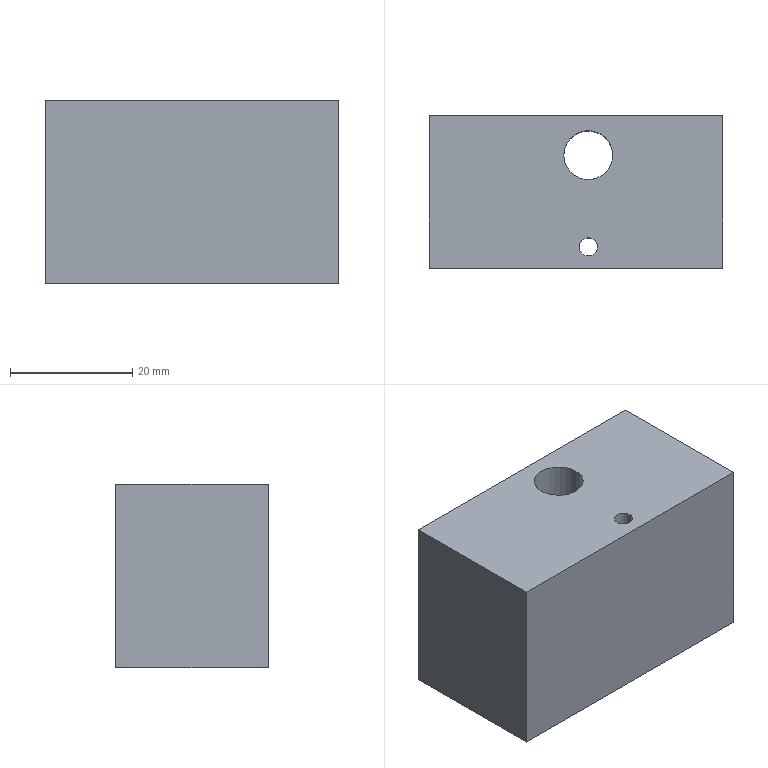Part | SolidWorks | features Cut 2, Extrusion 1, HoleWzd 1 | 1 solid | 22 faces | box 48 x 25 x 30 mm | volume 34166 mm3 | cylinder 10 | cone 6 | plane 6 | commonest cylinder face diameters 2.5 x6 3 x2 8 x2
STEP:
#1=CARTESIAN_POINT('',(12.5,17.5,-12.75));
#2=VERTEX_POINT('',#1);
#3=CARTESIAN_POINT('',(12.5,17.5,-10.25));
#4=VERTEX_POINT('',#3);
#5=CARTESIAN_POINT('',(12.5,17.5,-11.5));
#6=DIRECTION('',(0.,1.,0.));
#7=DIRECTION('',(0.,0.,1.));
#8=AXIS2_PLACEMENT_3D('',#5,#6,#7);
#9=CIRCLE('',#8,1.25);
#10=EDGE_CURVE('',#2,#4,#9,.T.);
#11=ORIENTED_EDGE('',*,*,#10,.F.);
#12=CARTESIAN_POINT('',(12.5,25.,-12.75));
#13=VERTEX_POINT('',#12);
#14=CARTESIAN_POINT('',(12.5,25.,-12.75));
#15=DIRECTION('',(0.,1.,0.));
#16=VECTOR('',#15,1000.);
#17=LINE('',#14,#16);
#18=EDGE_CURVE('',#2,#13,#17,.T.);
#19=ORIENTED_EDGE('',*,*,#18,.T.);
#20=CARTESIAN_POINT('',(12.5,25.,-10.25));
#21=VERTEX_POINT('',#20);
#22=CARTESIAN_POINT('',(12.5,25.,-11.5));
#23=DIRECTION('',(0.,1.,0.));
#24=DIRECTION('',(0.,0.,1.));
#25=AXIS2_PLACEMENT_3D('',#22,#23,#24);
#26=CIRCLE('',#25,1.25);
#27=EDGE_CURVE('',#13,#21,#26,.T.);
#28=ORIENTED_EDGE('',*,*,#27,.T.);
#29=CARTESIAN_POINT('',(12.5,25.,-10.25));
#30=DIRECTION('',(0.,1.,0.));
#31=VECTOR('',#30,1000.);
#32=LINE('',#29,#31);
#33=EDGE_CURVE('',#4,#21,#32,.T.);
#34=ORIENTED_EDGE('',*,*,#33,.F.);
#35=EDGE_LOOP('',(#11,#19,#28,#34));
#36=FACE_OUTER_BOUND('',#35,.T.);
#37=CARTESIAN_POINT('',(12.5,25.,-11.5));
#38=DIRECTION('',(0.,1.,0.));
#39=DIRECTION('',(0.,0.,1.));
#40=AXIS2_PLACEMENT_3D('',#37,#38,#39);
#41=CYLINDRICAL_SURFACE('',#40,1.25);
#42=ADVANCED_FACE('',(#36),#41,.F.);
#43=CARTESIAN_POINT('',(12.5,16.749,-11.5));
#44=VERTEX_POINT('',#43);
#45=CARTESIAN_POINT('',(12.5,17.5,-10.25));
#46=DIRECTION('',(0.,0.515,0.8572));
#47=VECTOR('',#46,1000.);
#48=LINE('',#45,#47);
#49=EDGE_CURVE('',#44,#4,#48,.T.);
#50=ORIENTED_EDGE('',*,*,#49,.F.);
#51=CARTESIAN_POINT('',(12.5,17.5,-12.75));
#52=DIRECTION('',(0.,0.515,-0.8572));
#53=VECTOR('',#52,1000.);
#54=LINE('',#51,#53);
#55=EDGE_CURVE('',#44,#2,#54,.T.);
#56=ORIENTED_EDGE('',*,*,#55,.T.);
#57=ORIENTED_EDGE('',*,*,#10,.T.);
#58=EDGE_LOOP('',(#50,#56,#57));
#59=FACE_OUTER_BOUND('',#58,.T.);
#60=CARTESIAN_POINT('',(12.5,17.5,-11.5));
#61=DIRECTION('',(0.,1.,0.));
#62=DIRECTION('',(0.,0.,1.));
#63=AXIS2_PLACEMENT_3D('',#60,#61,#62);
#64=CONICAL_SURFACE('',#63,1.25,1.03);
#65=ADVANCED_FACE('',(#59),#64,.F.);
#66=CARTESIAN_POINT('',(12.5,17.5,-1.25));
#67=VERTEX_POINT('',#66);
#68=CARTESIAN_POINT('',(12.5,17.5,1.25));
#69=VERTEX_POINT('',#68);
#70=CARTESIAN_POINT('',(12.5,17.5,0.));
#71=DIRECTION('',(0.,1.,0.));
#72=DIRECTION('',(0.,0.,1.));
#73=AXIS2_PLACEMENT_3D('',#70,#71,#72);
#74=CIRCLE('',#73,1.25);
#75=EDGE_CURVE('',#67,#69,#74,.T.);
#76=ORIENTED_EDGE('',*,*,#75,.F.);
#77=CARTESIAN_POINT('',(12.5,25.,-1.25));
#78=VERTEX_POINT('',#77);
#79=CARTESIAN_POINT('',(12.5,25.,-1.25));
#80=DIRECTION('',(0.,1.,0.));
#81=VECTOR('',#80,1000.);
#82=LINE('',#79,#81);
#83=EDGE_CURVE('',#67,#78,#82,.T.);
#84=ORIENTED_EDGE('',*,*,#83,.T.);
#85=CARTESIAN_POINT('',(12.5,25.,1.25));
#86=VERTEX_POINT('',#85);
#87=CARTESIAN_POINT('',(12.5,25.,0.));
#88=DIRECTION('',(0.,1.,0.));
#89=DIRECTION('',(0.,0.,1.));
#90=AXIS2_PLACEMENT_3D('',#87,#88,#89);
#91=CIRCLE('',#90,1.25);
#92=EDGE_CURVE('',#78,#86,#91,.T.);
#93=ORIENTED_EDGE('',*,*,#92,.T.);
#94=CARTESIAN_POINT('',(12.5,25.,1.25));
#95=DIRECTION('',(0.,1.,0.));
#96=VECTOR('',#95,1000.);
#97=LINE('',#94,#96);
#98=EDGE_CURVE('',#69,#86,#97,.T.);
#99=ORIENTED_EDGE('',*,*,#98,.F.);
#100=EDGE_LOOP('',(#76,#84,#93,#99));
#101=FACE_OUTER_BOUND('',#100,.T.);
#102=CARTESIAN_POINT('',(12.5,25.,0.));
#103=DIRECTION('',(0.,1.,0.));
#104=DIRECTION('',(0.,0.,1.));
#105=AXIS2_PLACEMENT_3D('',#102,#103,#104);
#106=CYLINDRICAL_SURFACE('',#105,1.25);
#107=ADVANCED_FACE('',(#101),#106,.F.);
#108=CARTESIAN_POINT('',(12.5,16.749,0.));
#109=VERTEX_POINT('',#108);
#110=CARTESIAN_POINT('',(12.5,17.5,1.25));
#111=DIRECTION('',(0.,0.515,0.8572));
#112=VECTOR('',#111,1000.);
#113=LINE('',#110,#112);
#114=EDGE_CURVE('',#109,#69,#113,.T.);
#115=ORIENTED_EDGE('',*,*,#114,.F.);
#116=CARTESIAN_POINT('',(12.5,17.5,-1.25));
#117=DIRECTION('',(0.,0.515,-0.8572));
#118=VECTOR('',#117,1000.);
#119=LINE('',#116,#118);
#120=EDGE_CURVE('',#109,#67,#119,.T.);
#121=ORIENTED_EDGE('',*,*,#120,.T.);
#122=ORIENTED_EDGE('',*,*,#75,.T.);
#123=EDGE_LOOP('',(#115,#121,#122));
#124=FACE_OUTER_BOUND('',#123,.T.);
#125=CARTESIAN_POINT('',(12.5,17.5,0.));
#126=DIRECTION('',(0.,1.,0.));
#127=DIRECTION('',(0.,0.,1.));
#128=AXIS2_PLACEMENT_3D('',#125,#126,#127);
#129=CONICAL_SURFACE('',#128,1.25,1.03);
#130=ADVANCED_FACE('',(#124),#129,.F.);
#131=CARTESIAN_POINT('',(12.5,17.5,10.25));
#132=VERTEX_POINT('',#131);
#133=CARTESIAN_POINT('',(12.5,17.5,12.75));
#134=VERTEX_POINT('',#133);
#135=CARTESIAN_POINT('',(12.5,17.5,11.5));
#136=DIRECTION('',(0.,1.,0.));
#137=DIRECTION('',(0.,0.,1.));
#138=AXIS2_PLACEMENT_3D('',#135,#136,#137);
#139=CIRCLE('',#138,1.25);
#140=EDGE_CURVE('',#132,#134,#139,.T.);
#141=ORIENTED_EDGE('',*,*,#140,.F.);
#142=CARTESIAN_POINT('',(12.5,25.,10.25));
#143=VERTEX_POINT('',#142);
#144=CARTESIAN_POINT('',(12.5,25.,10.25));
#145=DIRECTION('',(0.,1.,0.));
#146=VECTOR('',#145,1000.);
#147=LINE('',#144,#146);
#148=EDGE_CURVE('',#132,#143,#147,.T.);
#149=ORIENTED_EDGE('',*,*,#148,.T.);
#150=CARTESIAN_POINT('',(12.5,25.,12.75));
#151=VERTEX_POINT('',#150);
#152=CARTESIAN_POINT('',(12.5,25.,11.5));
#153=DIRECTION('',(0.,1.,0.));
#154=DIRECTION('',(0.,0.,1.));
#155=AXIS2_PLACEMENT_3D('',#152,#153,#154);
#156=CIRCLE('',#155,1.25);
#157=EDGE_CURVE('',#143,#151,#156,.T.);
#158=ORIENTED_EDGE('',*,*,#157,.T.);
#159=CARTESIAN_POINT('',(12.5,25.,12.75));
#160=DIRECTION('',(0.,1.,0.));
#161=VECTOR('',#160,1000.);
#162=LINE('',#159,#161);
#163=EDGE_CURVE('',#134,#151,#162,.T.);
#164=ORIENTED_EDGE('',*,*,#163,.F.);
#165=EDGE_LOOP('',(#141,#149,#158,#164));
#166=FACE_OUTER_BOUND('',#165,.T.);
#167=CARTESIAN_POINT('',(12.5,25.,11.5));
#168=DIRECTION('',(0.,1.,0.));
#169=DIRECTION('',(0.,0.,1.));
#170=AXIS2_PLACEMENT_3D('',#167,#168,#169);
#171=CYLINDRICAL_SURFACE('',#170,1.25);
#172=ADVANCED_FACE('',(#166),#171,.F.);
#173=CARTESIAN_POINT('',(12.5,16.749,11.5));
#174=VERTEX_POINT('',#173);
#175=CARTESIAN_POINT('',(12.5,17.5,12.75));
#176=DIRECTION('',(0.,0.515,0.8572));
#177=VECTOR('',#176,1000.);
#178=LINE('',#175,#177);
#179=EDGE_CURVE('',#174,#134,#178,.T.);
#180=ORIENTED_EDGE('',*,*,#179,.F.);
#181=CARTESIAN_POINT('',(12.5,17.5,10.25));
#182=DIRECTION('',(0.,0.515,-0.8572));
#183=VECTOR('',#182,1000.);
#184=LINE('',#181,#183);
#185=EDGE_CURVE('',#174,#132,#184,.T.);
#186=ORIENTED_EDGE('',*,*,#185,.T.);
#187=ORIENTED_EDGE('',*,*,#140,.T.);
#188=EDGE_LOOP('',(#180,#186,#187));
#189=FACE_OUTER_BOUND('',#188,.T.);
#190=CARTESIAN_POINT('',(12.5,17.5,11.5));
#191=DIRECTION('',(0.,1.,0.));
#192=DIRECTION('',(0.,0.,1.));
#193=AXIS2_PLACEMENT_3D('',#190,#191,#192);
#194=CONICAL_SURFACE('',#193,1.25,1.03);
#195=ADVANCED_FACE('',(#189),#194,.F.);
#196=CARTESIAN_POINT('',(6.,18.5,-15.));
#197=VERTEX_POINT('',#196);
#198=CARTESIAN_POINT('',(-2.,18.5,-15.));
#199=VERTEX_POINT('',#198);
#200=CARTESIAN_POINT('',(2.,18.5,-15.));
#201=DIRECTION('',(0.,0.,-1.));
#202=DIRECTION('',(1.,0.,0.));
#203=AXIS2_PLACEMENT_3D('',#200,#201,#202);
#204=CIRCLE('',#203,4.);
#205=EDGE_CURVE('',#197,#199,#204,.T.);
#206=ORIENTED_EDGE('',*,*,#205,.T.);
#207=CARTESIAN_POINT('',(-2.,18.5,15.));
#208=VERTEX_POINT('',#207);
#209=CARTESIAN_POINT('',(-2.,18.5,-15.001));
#210=DIRECTION('',(0.,0.,1.));
#211=VECTOR('',#210,1000.);
#212=LINE('',#209,#211);
#213=EDGE_CURVE('',#199,#208,#212,.T.);
#214=ORIENTED_EDGE('',*,*,#213,.T.);
#215=CARTESIAN_POINT('',(6.,18.5,15.));
#216=VERTEX_POINT('',#215);
#217=CARTESIAN_POINT('',(2.,18.5,15.));
#218=DIRECTION('',(0.,0.,1.));
#219=DIRECTION('',(1.,0.,0.));
#220=AXIS2_PLACEMENT_3D('',#217,#218,#219);
#221=CIRCLE('',#220,4.);
#222=EDGE_CURVE('',#208,#216,#221,.T.);
#223=ORIENTED_EDGE('',*,*,#222,.T.);
#224=CARTESIAN_POINT('',(6.,18.5,-15.001));
#225=DIRECTION('',(0.,0.,1.));
#226=VECTOR('',#225,1000.);
#227=LINE('',#224,#226);
#228=EDGE_CURVE('',#197,#216,#227,.T.);
#229=ORIENTED_EDGE('',*,*,#228,.F.);
#230=EDGE_LOOP('',(#206,#214,#223,#229));
#231=FACE_OUTER_BOUND('',#230,.T.);
#232=CARTESIAN_POINT('',(2.,18.5,-15.001));
#233=DIRECTION('',(0.,0.,1.));
#234=DIRECTION('',(1.,0.,0.));
#235=AXIS2_PLACEMENT_3D('',#232,#233,#234);
#236=CYLINDRICAL_SURFACE('',#235,4.);
#237=ADVANCED_FACE('',(#231),#236,.F.);
#238=CARTESIAN_POINT('',(3.5,3.5,-15.));
#239=VERTEX_POINT('',#238);
#240=CARTESIAN_POINT('',(0.5,3.5,-15.));
#241=VERTEX_POINT('',#240);
#242=CARTESIAN_POINT('',(2.,3.5,-15.));
#243=DIRECTION('',(0.,0.,-1.));
#244=DIRECTION('',(1.,0.,0.));
#245=AXIS2_PLACEMENT_3D('',#242,#243,#244);
#246=CIRCLE('',#245,1.5);
#247=EDGE_CURVE('',#239,#241,#246,.T.);
#248=ORIENTED_EDGE('',*,*,#247,.T.);
#249=CARTESIAN_POINT('',(0.5,3.5,15.));
#250=VERTEX_POINT('',#249);
#251=CARTESIAN_POINT('',(0.5,3.5,-15.001));
#252=DIRECTION('',(0.,0.,1.));
#253=VECTOR('',#252,1000.);
#254=LINE('',#251,#253);
#255=EDGE_CURVE('',#241,#250,#254,.T.);
#256=ORIENTED_EDGE('',*,*,#255,.T.);
#257=CARTESIAN_POINT('',(3.5,3.5,15.));
#258=VERTEX_POINT('',#257);
#259=CARTESIAN_POINT('',(2.,3.5,15.));
#260=DIRECTION('',(0.,0.,1.));
#261=DIRECTION('',(1.,0.,0.));
#262=AXIS2_PLACEMENT_3D('',#259,#260,#261);
#263=CIRCLE('',#262,1.5);
#264=EDGE_CURVE('',#250,#258,#263,.T.);
#265=ORIENTED_EDGE('',*,*,#264,.T.);
#266=CARTESIAN_POINT('',(3.5,3.5,-15.001));
#267=DIRECTION('',(0.,0.,1.));
#268=VECTOR('',#267,1000.);
#269=LINE('',#266,#268);
#270=EDGE_CURVE('',#239,#258,#269,.T.);
#271=ORIENTED_EDGE('',*,*,#270,.F.);
#272=EDGE_LOOP('',(#248,#256,#265,#271));
#273=FACE_OUTER_BOUND('',#272,.T.);
#274=CARTESIAN_POINT('',(2.,3.5,-15.001));
#275=DIRECTION('',(0.,0.,1.));
#276=DIRECTION('',(1.,0.,0.));
#277=AXIS2_PLACEMENT_3D('',#274,#275,#276);
#278=CYLINDRICAL_SURFACE('',#277,1.5);
#279=ADVANCED_FACE('',(#273),#278,.F.);
#280=CARTESIAN_POINT('',(24.,0.,15.));
#281=VERTEX_POINT('',#280);
#282=CARTESIAN_POINT('',(24.,0.,-15.));
#283=VERTEX_POINT('',#282);
#284=CARTESIAN_POINT('',(24.,0.,-15.));
#285=DIRECTION('',(0.,0.,-1.));
#286=VECTOR('',#285,1000.);
#287=LINE('',#284,#286);
#288=EDGE_CURVE('',#281,#283,#287,.T.);
#289=ORIENTED_EDGE('',*,*,#288,.T.);
#290=CARTESIAN_POINT('',(24.,25.,-15.));
#291=VERTEX_POINT('',#290);
#292=CARTESIAN_POINT('',(24.,25.,-15.));
#293=DIRECTION('',(0.,-1.,0.));
#294=VECTOR('',#293,1000.);
#295=LINE('',#292,#294);
#296=EDGE_CURVE('',#291,#283,#295,.T.);
#297=ORIENTED_EDGE('',*,*,#296,.F.);
#298=CARTESIAN_POINT('',(24.,25.,15.));
#299=VERTEX_POINT('',#298);
#300=CARTESIAN_POINT('',(24.,25.,-15.));
#301=DIRECTION('',(0.,0.,-1.));
#302=VECTOR('',#301,1000.);
#303=LINE('',#300,#302);
#304=EDGE_CURVE('',#299,#291,#303,.T.);
#305=ORIENTED_EDGE('',*,*,#304,.F.);
#306=CARTESIAN_POINT('',(24.,25.,15.));
#307=DIRECTION('',(0.,-1.,0.));
#308=VECTOR('',#307,1000.);
#309=LINE('',#306,#308);
#310=EDGE_CURVE('',#299,#281,#309,.T.);
#311=ORIENTED_EDGE('',*,*,#310,.T.);
#312=EDGE_LOOP('',(#289,#297,#305,#311));
#313=FACE_OUTER_BOUND('',#312,.T.);
#314=CARTESIAN_POINT('',(24.,25.,-15.));
#315=DIRECTION('',(-1.,0.,0.));
#316=DIRECTION('',(0.,0.,1.));
#317=AXIS2_PLACEMENT_3D('',#314,#315,#316);
#318=PLANE('',#317);
#319=ADVANCED_FACE('',(#313),#318,.F.);
#320=ORIENTED_EDGE('',*,*,#205,.F.);
#321=CARTESIAN_POINT('',(2.,18.5,-15.));
#322=DIRECTION('',(0.,0.,-1.));
#323=DIRECTION('',(1.,0.,0.));
#324=AXIS2_PLACEMENT_3D('',#321,#322,#323);
#325=CIRCLE('',#324,4.);
#326=EDGE_CURVE('',#199,#197,#325,.T.);
#327=ORIENTED_EDGE('',*,*,#326,.F.);
#328=EDGE_LOOP('',(#320,#327));
#329=FACE_BOUND('',#328,.T.);
#330=ORIENTED_EDGE('',*,*,#247,.F.);
#331=CARTESIAN_POINT('',(2.,3.5,-15.));
#332=DIRECTION('',(0.,0.,-1.));
#333=DIRECTION('',(1.,0.,0.));
#334=AXIS2_PLACEMENT_3D('',#331,#332,#333);
#335=CIRCLE('',#334,1.5);
#336=EDGE_CURVE('',#241,#239,#335,.T.);
#337=ORIENTED_EDGE('',*,*,#336,.F.);
#338=EDGE_LOOP('',(#330,#337));
#339=FACE_BOUND('',#338,.T.);
#340=CARTESIAN_POINT('',(-24.,0.,-15.));
#341=VERTEX_POINT('',#340);
#342=CARTESIAN_POINT('',(-24.,0.,-15.));
#343=DIRECTION('',(-1.,0.,0.));
#344=VECTOR('',#343,1000.);
#345=LINE('',#342,#344);
#346=EDGE_CURVE('',#283,#341,#345,.T.);
#347=ORIENTED_EDGE('',*,*,#346,.T.);
#348=CARTESIAN_POINT('',(-24.,25.,-15.));
#349=VERTEX_POINT('',#348);
#350=CARTESIAN_POINT('',(-24.,25.,-15.));
#351=DIRECTION('',(0.,-1.,0.));
#352=VECTOR('',#351,1000.);
#353=LINE('',#350,#352);
#354=EDGE_CURVE('',#349,#341,#353,.T.);
#355=ORIENTED_EDGE('',*,*,#354,.F.);
#356=CARTESIAN_POINT('',(-24.,25.,-15.));
#357=DIRECTION('',(-1.,0.,0.));
#358=VECTOR('',#357,1000.);
#359=LINE('',#356,#358);
#360=EDGE_CURVE('',#291,#349,#359,.T.);
#361=ORIENTED_EDGE('',*,*,#360,.F.);
#362=ORIENTED_EDGE('',*,*,#296,.T.);
#363=EDGE_LOOP('',(#347,#355,#361,#362));
#364=FACE_OUTER_BOUND('',#363,.T.);
#365=CARTESIAN_POINT('',(-24.,25.,-15.));
#366=DIRECTION('',(0.,0.,1.));
#367=DIRECTION('',(1.,0.,0.));
#368=AXIS2_PLACEMENT_3D('',#365,#366,#367);
#369=PLANE('',#368);
#370=ADVANCED_FACE('',(#329,#339,#364),#369,.F.);
#371=CARTESIAN_POINT('',(-24.,0.,15.));
#372=VERTEX_POINT('',#371);
#373=CARTESIAN_POINT('',(-24.,0.,-15.));
#374=DIRECTION('',(0.,0.,1.));
#375=VECTOR('',#374,1000.);
#376=LINE('',#373,#375);
#377=EDGE_CURVE('',#341,#372,#376,.T.);
#378=ORIENTED_EDGE('',*,*,#377,.T.);
#379=CARTESIAN_POINT('',(-24.,25.,15.));
#380=VERTEX_POINT('',#379);
#381=CARTESIAN_POINT('',(-24.,25.,15.));
#382=DIRECTION('',(0.,-1.,0.));
#383=VECTOR('',#382,1000.);
#384=LINE('',#381,#383);
#385=EDGE_CURVE('',#380,#372,#384,.T.);
#386=ORIENTED_EDGE('',*,*,#385,.F.);
#387=CARTESIAN_POINT('',(-24.,25.,-15.));
#388=DIRECTION('',(0.,0.,1.));
#389=VECTOR('',#388,1000.);
#390=LINE('',#387,#389);
#391=EDGE_CURVE('',#349,#380,#390,.T.);
#392=ORIENTED_EDGE('',*,*,#391,.F.);
#393=ORIENTED_EDGE('',*,*,#354,.T.);
#394=EDGE_LOOP('',(#378,#386,#392,#393));
#395=FACE_OUTER_BOUND('',#394,.T.);
#396=CARTESIAN_POINT('',(-24.,25.,-15.));
#397=DIRECTION('',(1.,0.,0.));
#398=DIRECTION('',(0.,0.,-1.));
#399=AXIS2_PLACEMENT_3D('',#396,#397,#398);
#400=PLANE('',#399);
#401=ADVANCED_FACE('',(#395),#400,.F.);
#402=CARTESIAN_POINT('',(2.,18.5,15.));
#403=DIRECTION('',(0.,0.,1.));
#404=DIRECTION('',(1.,0.,0.));
#405=AXIS2_PLACEMENT_3D('',#402,#403,#404);
#406=CIRCLE('',#405,4.);
#407=EDGE_CURVE('',#216,#208,#406,.T.);
#408=ORIENTED_EDGE('',*,*,#407,.F.);
#409=ORIENTED_EDGE('',*,*,#222,.F.);
#410=EDGE_LOOP('',(#408,#409));
#411=FACE_BOUND('',#410,.T.);
#412=CARTESIAN_POINT('',(2.,3.5,15.));
#413=DIRECTION('',(0.,0.,1.));
#414=DIRECTION('',(1.,0.,0.));
#415=AXIS2_PLACEMENT_3D('',#412,#413,#414);
#416=CIRCLE('',#415,1.5);
#417=EDGE_CURVE('',#258,#250,#416,.T.);
#418=ORIENTED_EDGE('',*,*,#417,.F.);
#419=ORIENTED_EDGE('',*,*,#264,.F.);
#420=EDGE_LOOP('',(#418,#419));
#421=FACE_BOUND('',#420,.T.);
#422=CARTESIAN_POINT('',(-24.,0.,15.));
#423=DIRECTION('',(1.,0.,0.));
#424=VECTOR('',#423,1000.);
#425=LINE('',#422,#424);
#426=EDGE_CURVE('',#372,#281,#425,.T.);
#427=ORIENTED_EDGE('',*,*,#426,.T.);
#428=ORIENTED_EDGE('',*,*,#310,.F.);
#429=CARTESIAN_POINT('',(-24.,25.,15.));
#430=DIRECTION('',(1.,0.,0.));
#431=VECTOR('',#430,1000.);
#432=LINE('',#429,#431);
#433=EDGE_CURVE('',#380,#299,#432,.T.);
#434=ORIENTED_EDGE('',*,*,#433,.F.);
#435=ORIENTED_EDGE('',*,*,#385,.T.);
#436=EDGE_LOOP('',(#427,#428,#434,#435));
#437=FACE_OUTER_BOUND('',#436,.T.);
#438=CARTESIAN_POINT('',(-24.,25.,15.));
#439=DIRECTION('',(0.,0.,-1.));
#440=DIRECTION('',(-1.,0.,0.));
#441=AXIS2_PLACEMENT_3D('',#438,#439,#440);
#442=PLANE('',#441);
#443=ADVANCED_FACE('',(#411,#421,#437),#442,.F.);
#444=CARTESIAN_POINT('',(12.5,25.,-11.5));
#445=DIRECTION('',(0.,1.,0.));
#446=DIRECTION('',(0.,0.,1.));
#447=AXIS2_PLACEMENT_3D('',#444,#445,#446);
#448=CIRCLE('',#447,1.25);
#449=EDGE_CURVE('',#21,#13,#448,.T.);
#450=ORIENTED_EDGE('',*,*,#449,.F.);
#451=ORIENTED_EDGE('',*,*,#27,.F.);
#452=EDGE_LOOP('',(#450,#451));
#453=FACE_BOUND('',#452,.T.);
#454=CARTESIAN_POINT('',(12.5,25.,0.));
#455=DIRECTION('',(0.,1.,0.));
#456=DIRECTION('',(0.,0.,1.));
#457=AXIS2_PLACEMENT_3D('',#454,#455,#456);
#458=CIRCLE('',#457,1.25);
#459=EDGE_CURVE('',#86,#78,#458,.T.);
#460=ORIENTED_EDGE('',*,*,#459,.F.);
#461=ORIENTED_EDGE('',*,*,#92,.F.);
#462=EDGE_LOOP('',(#460,#461));
#463=FACE_BOUND('',#462,.T.);
#464=CARTESIAN_POINT('',(12.5,25.,11.5));
#465=DIRECTION('',(0.,1.,0.));
#466=DIRECTION('',(0.,0.,1.));
#467=AXIS2_PLACEMENT_3D('',#464,#465,#466);
#468=CIRCLE('',#467,1.25);
#469=EDGE_CURVE('',#151,#143,#468,.T.);
#470=ORIENTED_EDGE('',*,*,#469,.F.);
#471=ORIENTED_EDGE('',*,*,#157,.F.);
#472=EDGE_LOOP('',(#470,#471));
#473=FACE_BOUND('',#472,.T.);
#474=ORIENTED_EDGE('',*,*,#304,.T.);
#475=ORIENTED_EDGE('',*,*,#360,.T.);
#476=ORIENTED_EDGE('',*,*,#391,.T.);
#477=ORIENTED_EDGE('',*,*,#433,.T.);
#478=EDGE_LOOP('',(#474,#475,#476,#477));
#479=FACE_OUTER_BOUND('',#478,.T.);
#480=CARTESIAN_POINT('',(0.,25.,0.));
#481=DIRECTION('',(0.,1.,0.));
#482=DIRECTION('',(0.,0.,1.));
#483=AXIS2_PLACEMENT_3D('',#480,#481,#482);
#484=PLANE('',#483);
#485=ADVANCED_FACE('',(#453,#463,#473,#479),#484,.T.);
#486=ORIENTED_EDGE('',*,*,#288,.F.);
#487=ORIENTED_EDGE('',*,*,#426,.F.);
#488=ORIENTED_EDGE('',*,*,#377,.F.);
#489=ORIENTED_EDGE('',*,*,#346,.F.);
#490=EDGE_LOOP('',(#486,#487,#488,#489));
#491=FACE_OUTER_BOUND('',#490,.T.);
#492=CARTESIAN_POINT('',(0.,0.,0.));
#493=DIRECTION('',(0.,1.,0.));
#494=DIRECTION('',(0.,0.,1.));
#495=AXIS2_PLACEMENT_3D('',#492,#493,#494);
#496=PLANE('',#495);
#497=ADVANCED_FACE('',(#491),#496,.F.);
#498=ORIENTED_EDGE('',*,*,#255,.F.);
#499=ORIENTED_EDGE('',*,*,#336,.T.);
#500=ORIENTED_EDGE('',*,*,#270,.T.);
#501=ORIENTED_EDGE('',*,*,#417,.T.);
#502=EDGE_LOOP('',(#498,#499,#500,#501));
#503=FACE_OUTER_BOUND('',#502,.T.);
#504=CARTESIAN_POINT('',(2.,3.5,-15.001));
#505=DIRECTION('',(0.,0.,1.));
#506=DIRECTION('',(1.,0.,0.));
#507=AXIS2_PLACEMENT_3D('',#504,#505,#506);
#508=CYLINDRICAL_SURFACE('',#507,1.5);
#509=ADVANCED_FACE('',(#503),#508,.F.);
#510=ORIENTED_EDGE('',*,*,#213,.F.);
#511=ORIENTED_EDGE('',*,*,#326,.T.);
#512=ORIENTED_EDGE('',*,*,#228,.T.);
#513=ORIENTED_EDGE('',*,*,#407,.T.);
#514=EDGE_LOOP('',(#510,#511,#512,#513));
#515=FACE_OUTER_BOUND('',#514,.T.);
#516=CARTESIAN_POINT('',(2.,18.5,-15.001));
#517=DIRECTION('',(0.,0.,1.));
#518=DIRECTION('',(1.,0.,0.));
#519=AXIS2_PLACEMENT_3D('',#516,#517,#518);
#520=CYLINDRICAL_SURFACE('',#519,4.);
#521=ADVANCED_FACE('',(#515),#520,.F.);
#522=ORIENTED_EDGE('',*,*,#185,.F.);
#523=ORIENTED_EDGE('',*,*,#179,.T.);
#524=CARTESIAN_POINT('',(12.5,17.5,11.5));
#525=DIRECTION('',(0.,1.,0.));
#526=DIRECTION('',(0.,0.,1.));
#527=AXIS2_PLACEMENT_3D('',#524,#525,#526);
#528=CIRCLE('',#527,1.25);
#529=EDGE_CURVE('',#134,#132,#528,.T.);
#530=ORIENTED_EDGE('',*,*,#529,.T.);
#531=EDGE_LOOP('',(#522,#523,#530));
#532=FACE_OUTER_BOUND('',#531,.T.);
#533=CARTESIAN_POINT('',(12.5,17.5,11.5));
#534=DIRECTION('',(0.,1.,0.));
#535=DIRECTION('',(0.,0.,1.));
#536=AXIS2_PLACEMENT_3D('',#533,#534,#535);
#537=CONICAL_SURFACE('',#536,1.25,1.03);
#538=ADVANCED_FACE('',(#532),#537,.F.);
#539=ORIENTED_EDGE('',*,*,#148,.F.);
#540=ORIENTED_EDGE('',*,*,#529,.F.);
#541=ORIENTED_EDGE('',*,*,#163,.T.);
#542=ORIENTED_EDGE('',*,*,#469,.T.);
#543=EDGE_LOOP('',(#539,#540,#541,#542));
#544=FACE_OUTER_BOUND('',#543,.T.);
#545=CARTESIAN_POINT('',(12.5,25.,11.5));
#546=DIRECTION('',(0.,1.,0.));
#547=DIRECTION('',(0.,0.,1.));
#548=AXIS2_PLACEMENT_3D('',#545,#546,#547);
#549=CYLINDRICAL_SURFACE('',#548,1.25);
#550=ADVANCED_FACE('',(#544),#549,.F.);
#551=ORIENTED_EDGE('',*,*,#120,.F.);
#552=ORIENTED_EDGE('',*,*,#114,.T.);
#553=CARTESIAN_POINT('',(12.5,17.5,0.));
#554=DIRECTION('',(0.,1.,0.));
#555=DIRECTION('',(0.,0.,1.));
#556=AXIS2_PLACEMENT_3D('',#553,#554,#555);
#557=CIRCLE('',#556,1.25);
#558=EDGE_CURVE('',#69,#67,#557,.T.);
#559=ORIENTED_EDGE('',*,*,#558,.T.);
#560=EDGE_LOOP('',(#551,#552,#559));
#561=FACE_OUTER_BOUND('',#560,.T.);
#562=CARTESIAN_POINT('',(12.5,17.5,0.));
#563=DIRECTION('',(0.,1.,0.));
#564=DIRECTION('',(0.,0.,1.));
#565=AXIS2_PLACEMENT_3D('',#562,#563,#564);
#566=CONICAL_SURFACE('',#565,1.25,1.03);
#567=ADVANCED_FACE('',(#561),#566,.F.);
#568=ORIENTED_EDGE('',*,*,#83,.F.);
#569=ORIENTED_EDGE('',*,*,#558,.F.);
#570=ORIENTED_EDGE('',*,*,#98,.T.);
#571=ORIENTED_EDGE('',*,*,#459,.T.);
#572=EDGE_LOOP('',(#568,#569,#570,#571));
#573=FACE_OUTER_BOUND('',#572,.T.);
#574=CARTESIAN_POINT('',(12.5,25.,0.));
#575=DIRECTION('',(0.,1.,0.));
#576=DIRECTION('',(0.,0.,1.));
#577=AXIS2_PLACEMENT_3D('',#574,#575,#576);
#578=CYLINDRICAL_SURFACE('',#577,1.25);
#579=ADVANCED_FACE('',(#573),#578,.F.);
#580=ORIENTED_EDGE('',*,*,#55,.F.);
#581=ORIENTED_EDGE('',*,*,#49,.T.);
#582=CARTESIAN_POINT('',(12.5,17.5,-11.5));
#583=DIRECTION('',(0.,1.,0.));
#584=DIRECTION('',(0.,0.,1.));
#585=AXIS2_PLACEMENT_3D('',#582,#583,#584);
#586=CIRCLE('',#585,1.25);
#587=EDGE_CURVE('',#4,#2,#586,.T.);
#588=ORIENTED_EDGE('',*,*,#587,.T.);
#589=EDGE_LOOP('',(#580,#581,#588));
#590=FACE_OUTER_BOUND('',#589,.T.);
#591=CARTESIAN_POINT('',(12.5,17.5,-11.5));
#592=DIRECTION('',(0.,1.,0.));
#593=DIRECTION('',(0.,0.,1.));
#594=AXIS2_PLACEMENT_3D('',#591,#592,#593);
#595=CONICAL_SURFACE('',#594,1.25,1.03);
#596=ADVANCED_FACE('',(#590),#595,.F.);
#597=ORIENTED_EDGE('',*,*,#18,.F.);
#598=ORIENTED_EDGE('',*,*,#587,.F.);
#599=ORIENTED_EDGE('',*,*,#33,.T.);
#600=ORIENTED_EDGE('',*,*,#449,.T.);
#601=EDGE_LOOP('',(#597,#598,#599,#600));
#602=FACE_OUTER_BOUND('',#601,.T.);
#603=CARTESIAN_POINT('',(12.5,25.,-11.5));
#604=DIRECTION('',(0.,1.,0.));
#605=DIRECTION('',(0.,0.,1.));
#606=AXIS2_PLACEMENT_3D('',#603,#604,#605);
#607=CYLINDRICAL_SURFACE('',#606,1.25);
#608=ADVANCED_FACE('',(#602),#607,.F.);
#609=CLOSED_SHELL('',(#42,#65,#107,#130,#172,#195,#237,#279,#319,#370,#401,#443,#485,#497,#509,#521,#538,#550,#567,#579,#596,#608));
#610=MANIFOLD_SOLID_BREP('',#609);
#611=CARTESIAN_POINT('',(0.,0.,0.));
#612=DIRECTION('',(0.,0.,1.));
#613=DIRECTION('',(1.,0.,0.));
#614=AXIS2_PLACEMENT_3D('',#611,#612,#613);
#615=(LENGTH_UNIT()NAMED_UNIT(*)SI_UNIT(.MILLI.,.METRE.));
#616=UNCERTAINTY_MEASURE_WITH_UNIT(LENGTH_MEASURE(0.00001),#615,'','');
#617=(NAMED_UNIT(*)PLANE_ANGLE_UNIT()SI_UNIT($,.RADIAN.));
#618=(NAMED_UNIT(*)SI_UNIT($,.STERADIAN.)SOLID_ANGLE_UNIT());
#619=(GEOMETRIC_REPRESENTATION_CONTEXT(3)GLOBAL_UNCERTAINTY_ASSIGNED_CONTEXT((#616))GLOBAL_UNIT_ASSIGNED_CONTEXT((#615,#617,#618))REPRESENTATION_CONTEXT('',''));
#620=ADVANCED_BREP_SHAPE_REPRESENTATION('',(#610,#614),#619);